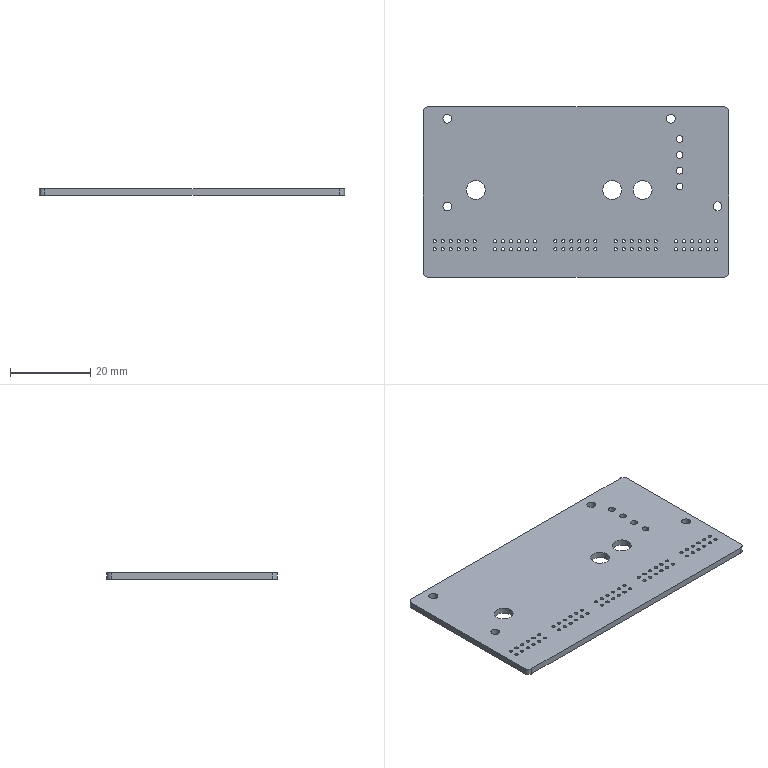Part | STEP file | Control module PCB | 1 solid | 81 faces | box 76.14 x 42.52 x 1.6 mm | volume 5007 mm3 | cylinder 75 | plane 6 | commonest cylinder face diameters 0.8 x60 1.7 x4 2.2 x4 2.54 x4 4.7 x3